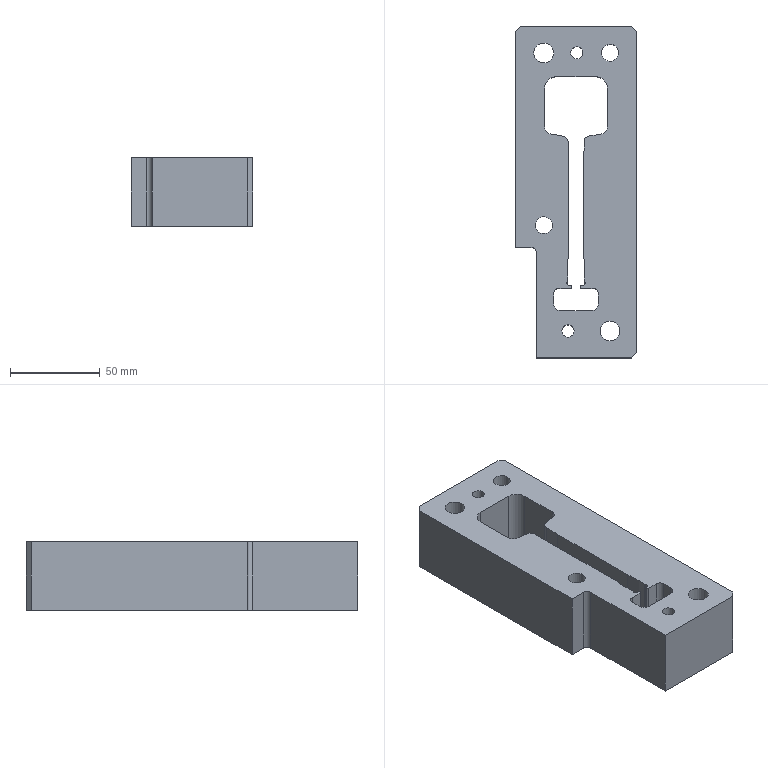Part | STEP file | 1_id178_x_t | 1 solid | 59 faces | box 68 x 185 x 38.1 mm | volume 347953 mm3 | cylinder 30 | plane 29 | commonest cylinder face diameters 6 x5 1.5 x4 3 x4 8 x4 6.8 x2 9.525 x2